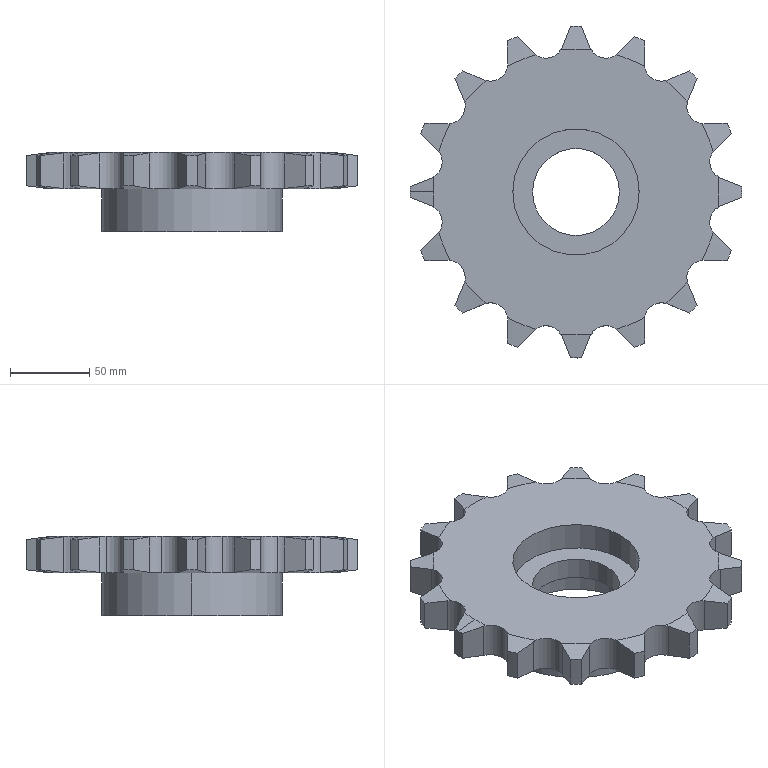Part | STEP file | 24A16T sprocket XG | 1 solid | 118 faces | box 210 x 210 x 50 mm | volume 700498 mm3 | cylinder 47 | plane 37 | cone 34 | commonest cylinder face diameters 22 x22 210 x17 80 x4 55 x2 114 x2